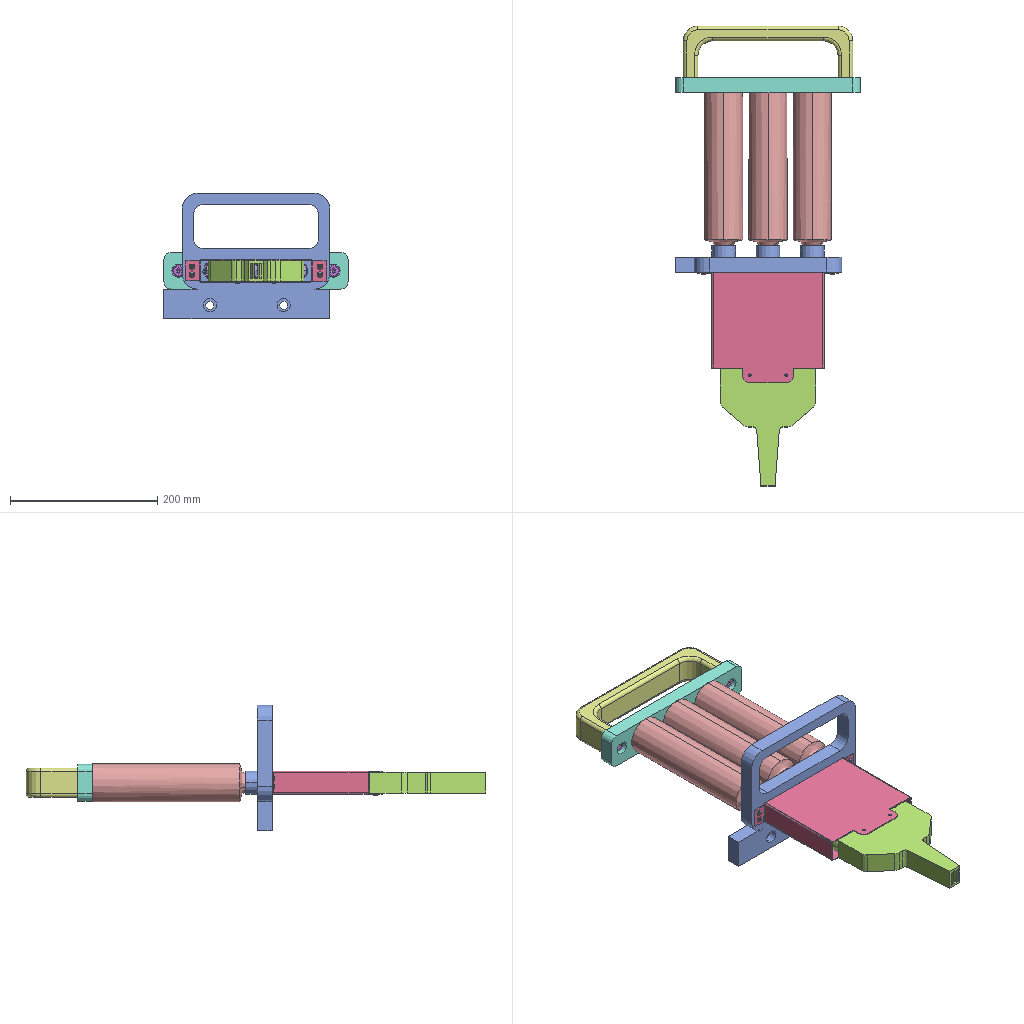Assembly | SolidWorks | 11 different items | 20 placed | box 250 x 624 x 170 mm
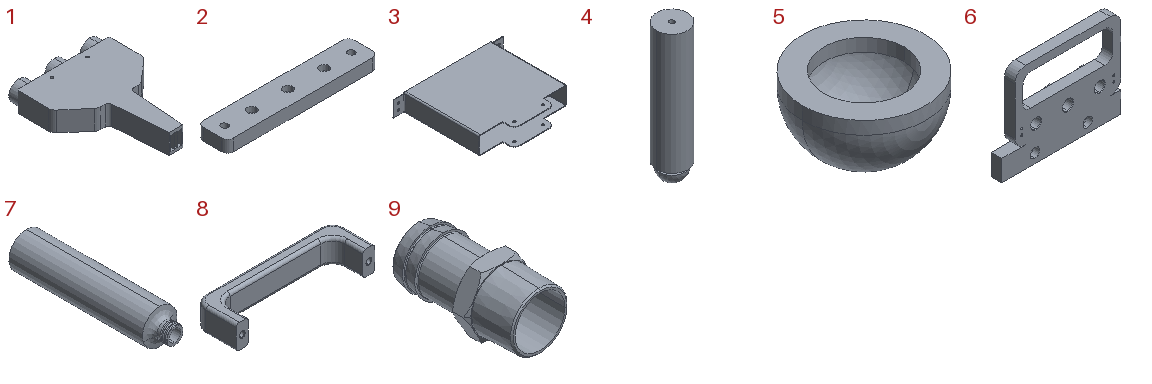Parts list (item | name | quantity | size | volume | features):
1 | - | x1 | 130 x 172 x 28 mm | 273655 mm3 | features MirrorPattern 5, ICE 4, Cut 3, Fillet 3, SweepCut 3, 3DProfileFeature 2, HoleWzd 2, Blend 1, Chamfer 1, CombineBodies 1, Extrusion 1, LPattern 1
2 | - | x1 | 250 x 50 x 20 mm | 234104 mm3 | features 3DProfileFeature 2, HoleWzd 2, Extrusion 1, Fillet 1, LPattern 1
3 | - | x1 | 190 x 150 x 31.2 mm | 60149 mm3 | features EdgeFlange 4, Cut 3, Fillet 1, FlatPattern 1, MirrorPattern 1, SMBaseFlange 1, SheetMetal 1
4 | - | x3 | 45.5 x 45.5 x 200 mm | 302158 mm3 | features 3DProfileFeature 1, HoleWzd 1, SavedExtBody 1
5 | - | x3 | 46 x 46 x 27.8 mm | 15701 mm3 | features SavedExtBody 1
6 | - | x1 | 225 x 37.797 x 170 mm | 483949 mm3 | features Fillet 4, ICE 4, Cut 3, HoleWzd 3, LPattern 3, 3DProfileFeature 2, Extrusion 1, Helix 1, SweepCut 1
7 | - | x3 | 52.001 x 224.797 x 52 mm | 100616 mm3 | features Blend 1, Helix 1, ICE 1, Revolution 1, Shell 1, Sweep 1
8 | - | x1 | 230 x 70 x 40 mm | 254336 mm3 | features Fillet 2, 3DProfileFeature 1, Extrusion 1, HoleWzd 1
9 | - | x4 | 25.403 x 44 x 22 mm | 3954 mm3 | features BaseBody 1
10 | hex lobular socket head cap screws-8.8 gb | x1 | - | - | -
11 | hexagon socket button head screws gb | x1 | - | - | -
Mates (type | each side: item.copy, entity, surface, feature):
Concentric | 7.1 face cylinder Boss-Extrude2 | 6.1 face cylinder Boss-Extrude3
Concentric | 7.1 edge | 6.1 edge
Coincident | 7.1 edge | 6.1 face plane Boss-Extrude3
Concentric | 7.2 face cylinder Boss-Extrude2 | 6.1 face cylinder LPattern2
Concentric | 2.1 face cylinder CBORE for M8 Hexagon socket head cap screws1 | 4.1 face cylinder Base Part-Part4^Auto Recover Assembly1-1
Coincident | 2.1 face plane Boss-Extrude1 | 4.1 face plane Base Part-Part4^Auto Recover Assembly1-1
Concentric | 4.1 face cylinder Base Part-Part4^Auto Recover Assembly1-1 | 5.1 face cylinder Base Part-Part4^Assembly1-1
DistanceDim | 5.1 face plane Base Part-Part4^Assembly1-1 | 4.1 face plane Base Part-Part4^Auto Recover Assembly1-1
DistanceDim | 1.1 face plane Boss-Extrude1 | 6.1 face plane Boss-Extrude1
Width | 6.1 face plane Boss-Extrude1 | 6.1 face plane Boss-Extrude1 | 3.1 face plane Edge-Flange1 | 3.1 face plane Edge-Flange1
Width | 6.1 face plane Boss-Extrude1 | 6.1 face plane Boss-Extrude1 | 1.1 face plane Cut-Extrude1 | 1.1 face plane Mirror2
Concentric | 7.1 face cylinder Revolve1 | 4.1 face cylinder Base Part-Part4^Auto Recover Assembly1-1
Coincident | 7.1 face plane Revolve1 | 2.1 face plane Boss-Extrude1
Concentric | 6.1 edge | 9.1 face cone Input1
Coincident | 6.1 face plane Boss-Extrude1 | 9.1 face plane Input1
Concentric | 1.1 face cylinder Loft1 | 9.2 face cylinder Input1
Concentric | 1.1 face cylinder G1/2 Tapped Hole1 | 9.2 face cone Input1
Coincident | 1.1 face plane Loft1 | 9.2 face plane Input1
Coincident | 6.1 face plane Boss-Extrude1 | 3.1 face plane Edge-Flange10